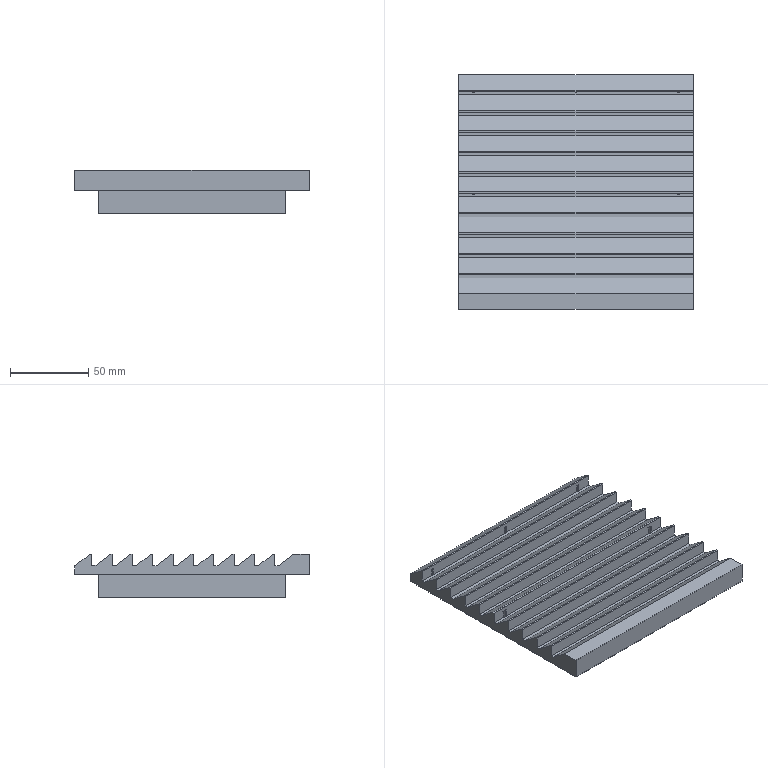Part | STEP file | Class B ventilation filter set ZL-803 (7032 glue) | 1 solid | 100 faces | box 150 x 150 x 28 mm | volume 421271 mm3 | plane 52 | cylinder 24 | cone 24 | commonest cylinder face diameters 3.3 x24